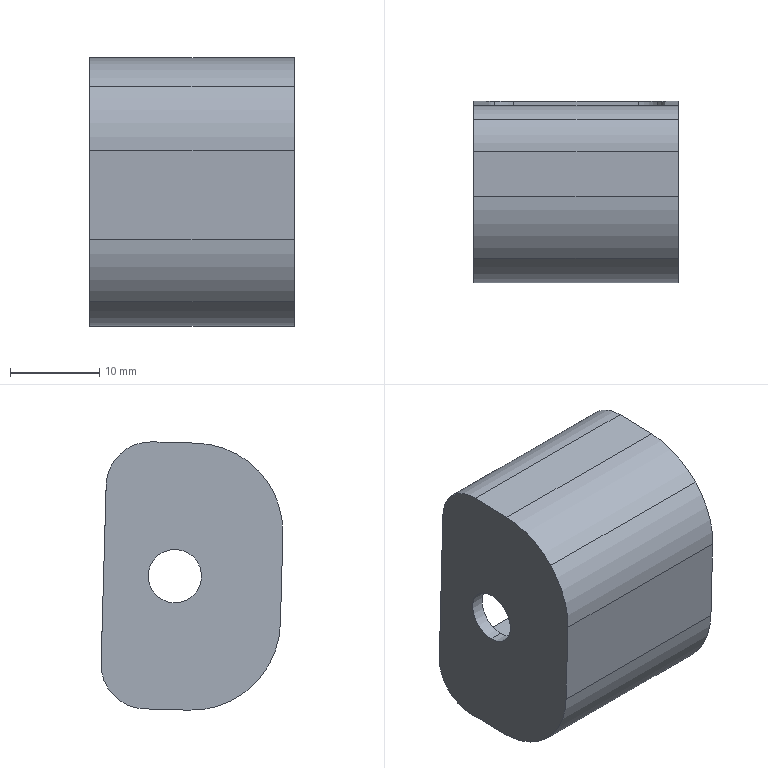Part | SolidWorks | features BaseBody 1 | 1 solid | 32 faces | box 23 x 20.424 x 30.136 mm | volume 5420 mm3 | cylinder 20 | plane 12 | commonest cylinder face diameters 6 x12 10 x4 20 x4
STEP:
#1=CARTESIAN_POINT('',(-20.895,-36.073,-245.05));
#2=VERTEX_POINT('',#1);
#3=CARTESIAN_POINT('',(-21.773,-36.013,-247.171));
#4=VERTEX_POINT('',#3);
#5=CARTESIAN_POINT('',(-18.773,-36.013,-247.171));
#6=DIRECTION('',(0.,-0.9996,-0.02838));
#7=DIRECTION('',(-0.7071,-0.02007,0.7068));
#8=AXIS2_PLACEMENT_3D('',#5,#6,#7);
#9=CIRCLE('',#8,3.);
#10=EDGE_CURVE('',#2,#4,#9,.T.);
#11=ORIENTED_EDGE('',*,*,#10,.F.);
#12=CARTESIAN_POINT('',(-20.895,-54.066,-245.561));
#13=VERTEX_POINT('',#12);
#14=CARTESIAN_POINT('',(-20.895,-36.073,-245.05));
#15=DIRECTION('',(0.,-0.9996,-0.02838));
#16=VECTOR('',#15,1000.);
#17=LINE('',#14,#16);
#18=EDGE_CURVE('',#2,#13,#17,.T.);
#19=ORIENTED_EDGE('',*,*,#18,.T.);
#20=CARTESIAN_POINT('',(-21.773,-54.005,-247.682));
#21=VERTEX_POINT('',#20);
#22=CARTESIAN_POINT('',(-18.773,-54.005,-247.682));
#23=DIRECTION('',(0.,0.9996,0.02838));
#24=DIRECTION('',(-0.7071,-0.02007,0.7068));
#25=AXIS2_PLACEMENT_3D('',#22,#23,#24);
#26=CIRCLE('',#25,3.);
#27=EDGE_CURVE('',#21,#13,#26,.T.);
#28=ORIENTED_EDGE('',*,*,#27,.F.);
#29=CARTESIAN_POINT('',(-21.773,-36.013,-247.171));
#30=DIRECTION('',(0.,0.9996,0.02838));
#31=VECTOR('',#30,1000.);
#32=LINE('',#29,#31);
#33=EDGE_CURVE('',#21,#4,#32,.T.);
#34=ORIENTED_EDGE('',*,*,#33,.T.);
#35=EDGE_LOOP('',(#11,#19,#28,#34));
#36=FACE_OUTER_BOUND('',#35,.T.);
#37=CARTESIAN_POINT('',(-18.773,-36.013,-247.171));
#38=DIRECTION('',(0.,-0.9996,-0.02838));
#39=DIRECTION('',(-0.7071,-0.02007,0.7068));
#40=AXIS2_PLACEMENT_3D('',#37,#38,#39);
#41=CYLINDRICAL_SURFACE('',#40,3.);
#42=ADVANCED_FACE('',(#36),#41,.F.);
#43=CARTESIAN_POINT('',(-2.652,-36.073,-245.05));
#44=VERTEX_POINT('',#43);
#45=CARTESIAN_POINT('',(-4.773,-36.098,-244.172));
#46=VERTEX_POINT('',#45);
#47=CARTESIAN_POINT('',(-4.773,-36.013,-247.171));
#48=DIRECTION('',(0.,-0.9996,-0.02838));
#49=DIRECTION('',(0.7071,-0.02007,0.7068));
#50=AXIS2_PLACEMENT_3D('',#47,#48,#49);
#51=CIRCLE('',#50,3.);
#52=EDGE_CURVE('',#44,#46,#51,.T.);
#53=ORIENTED_EDGE('',*,*,#52,.F.);
#54=CARTESIAN_POINT('',(-2.652,-54.066,-245.561));
#55=VERTEX_POINT('',#54);
#56=CARTESIAN_POINT('',(-2.652,-36.073,-245.05));
#57=DIRECTION('',(0.,-0.9996,-0.02838));
#58=VECTOR('',#57,1000.);
#59=LINE('',#56,#58);
#60=EDGE_CURVE('',#44,#55,#59,.T.);
#61=ORIENTED_EDGE('',*,*,#60,.T.);
#62=CARTESIAN_POINT('',(-4.773,-54.091,-244.683));
#63=VERTEX_POINT('',#62);
#64=CARTESIAN_POINT('',(-4.773,-54.005,-247.682));
#65=DIRECTION('',(0.,0.9996,0.02838));
#66=DIRECTION('',(0.7071,-0.02007,0.7068));
#67=AXIS2_PLACEMENT_3D('',#64,#65,#66);
#68=CIRCLE('',#67,3.);
#69=EDGE_CURVE('',#63,#55,#68,.T.);
#70=ORIENTED_EDGE('',*,*,#69,.F.);
#71=CARTESIAN_POINT('',(-4.773,-36.098,-244.172));
#72=DIRECTION('',(0.,0.9996,0.02838));
#73=VECTOR('',#72,1000.);
#74=LINE('',#71,#73);
#75=EDGE_CURVE('',#63,#46,#74,.T.);
#76=ORIENTED_EDGE('',*,*,#75,.T.);
#77=EDGE_LOOP('',(#53,#61,#70,#76));
#78=FACE_OUTER_BOUND('',#77,.T.);
#79=CARTESIAN_POINT('',(-4.773,-36.013,-247.171));
#80=DIRECTION('',(0.,-0.9996,-0.02838));
#81=DIRECTION('',(0.7071,-0.02007,0.7068));
#82=AXIS2_PLACEMENT_3D('',#79,#80,#81);
#83=CYLINDRICAL_SURFACE('',#82,3.);
#84=ADVANCED_FACE('',(#78),#83,.F.);
#85=CARTESIAN_POINT('',(-2.652,-35.555,-263.286));
#86=VERTEX_POINT('',#85);
#87=CARTESIAN_POINT('',(-1.773,-35.615,-261.165));
#88=VERTEX_POINT('',#87);
#89=CARTESIAN_POINT('',(-4.773,-35.615,-261.165));
#90=DIRECTION('',(0.,-0.9996,-0.02838));
#91=DIRECTION('',(0.7071,0.02007,-0.7068));
#92=AXIS2_PLACEMENT_3D('',#89,#90,#91);
#93=CIRCLE('',#92,3.);
#94=EDGE_CURVE('',#86,#88,#93,.T.);
#95=ORIENTED_EDGE('',*,*,#94,.F.);
#96=CARTESIAN_POINT('',(-2.652,-53.548,-263.797));
#97=VERTEX_POINT('',#96);
#98=CARTESIAN_POINT('',(-2.652,-35.555,-263.286));
#99=DIRECTION('',(0.,-0.9996,-0.02838));
#100=VECTOR('',#99,1000.);
#101=LINE('',#98,#100);
#102=EDGE_CURVE('',#86,#97,#101,.T.);
#103=ORIENTED_EDGE('',*,*,#102,.T.);
#104=CARTESIAN_POINT('',(-1.773,-53.608,-261.676));
#105=VERTEX_POINT('',#104);
#106=CARTESIAN_POINT('',(-4.773,-53.608,-261.676));
#107=DIRECTION('',(0.,0.9996,0.02838));
#108=DIRECTION('',(0.7071,0.02007,-0.7068));
#109=AXIS2_PLACEMENT_3D('',#106,#107,#108);
#110=CIRCLE('',#109,3.);
#111=EDGE_CURVE('',#105,#97,#110,.T.);
#112=ORIENTED_EDGE('',*,*,#111,.F.);
#113=CARTESIAN_POINT('',(-1.773,-35.615,-261.165));
#114=DIRECTION('',(0.,0.9996,0.02838));
#115=VECTOR('',#114,1000.);
#116=LINE('',#113,#115);
#117=EDGE_CURVE('',#105,#88,#116,.T.);
#118=ORIENTED_EDGE('',*,*,#117,.T.);
#119=EDGE_LOOP('',(#95,#103,#112,#118));
#120=FACE_OUTER_BOUND('',#119,.T.);
#121=CARTESIAN_POINT('',(-4.773,-35.615,-261.165));
#122=DIRECTION('',(0.,-0.9996,-0.02838));
#123=DIRECTION('',(0.7071,0.02007,-0.7068));
#124=AXIS2_PLACEMENT_3D('',#121,#122,#123);
#125=CYLINDRICAL_SURFACE('',#124,3.);
#126=ADVANCED_FACE('',(#120),#125,.F.);
#127=CARTESIAN_POINT('',(-20.895,-35.555,-263.286));
#128=VERTEX_POINT('',#127);
#129=CARTESIAN_POINT('',(-18.773,-35.53,-264.164));
#130=VERTEX_POINT('',#129);
#131=CARTESIAN_POINT('',(-18.773,-35.615,-261.165));
#132=DIRECTION('',(0.,-0.9996,-0.02838));
#133=DIRECTION('',(-0.7071,0.02007,-0.7068));
#134=AXIS2_PLACEMENT_3D('',#131,#132,#133);
#135=CIRCLE('',#134,3.);
#136=EDGE_CURVE('',#128,#130,#135,.T.);
#137=ORIENTED_EDGE('',*,*,#136,.F.);
#138=CARTESIAN_POINT('',(-20.895,-53.548,-263.797));
#139=VERTEX_POINT('',#138);
#140=CARTESIAN_POINT('',(-20.895,-35.555,-263.286));
#141=DIRECTION('',(0.,-0.9996,-0.02838));
#142=VECTOR('',#141,1000.);
#143=LINE('',#140,#142);
#144=EDGE_CURVE('',#128,#139,#143,.T.);
#145=ORIENTED_EDGE('',*,*,#144,.T.);
#146=CARTESIAN_POINT('',(-18.773,-53.523,-264.675));
#147=VERTEX_POINT('',#146);
#148=CARTESIAN_POINT('',(-18.773,-53.608,-261.676));
#149=DIRECTION('',(0.,0.9996,0.02838));
#150=DIRECTION('',(-0.7071,0.02007,-0.7068));
#151=AXIS2_PLACEMENT_3D('',#148,#149,#150);
#152=CIRCLE('',#151,3.);
#153=EDGE_CURVE('',#147,#139,#152,.T.);
#154=ORIENTED_EDGE('',*,*,#153,.F.);
#155=CARTESIAN_POINT('',(-18.773,-35.53,-264.164));
#156=DIRECTION('',(0.,0.9996,0.02838));
#157=VECTOR('',#156,1000.);
#158=LINE('',#155,#157);
#159=EDGE_CURVE('',#147,#130,#158,.T.);
#160=ORIENTED_EDGE('',*,*,#159,.T.);
#161=EDGE_LOOP('',(#137,#145,#154,#160));
#162=FACE_OUTER_BOUND('',#161,.T.);
#163=CARTESIAN_POINT('',(-18.773,-35.615,-261.165));
#164=DIRECTION('',(0.,-0.9996,-0.02838));
#165=DIRECTION('',(-0.7071,0.02007,-0.7068));
#166=AXIS2_PLACEMENT_3D('',#163,#164,#165);
#167=CYLINDRICAL_SURFACE('',#166,3.);
#168=ADVANCED_FACE('',(#162),#167,.F.);
#169=CARTESIAN_POINT('',(-0.2734,-43.726,-257.394));
#170=VERTEX_POINT('',#169);
#171=CARTESIAN_POINT('',(-0.2734,-43.896,-251.396));
#172=VERTEX_POINT('',#171);
#173=CARTESIAN_POINT('',(-0.2734,-43.811,-254.395));
#174=DIRECTION('',(-1.,0.,0.));
#175=DIRECTION('',(0.,-0.02838,0.9996));
#176=AXIS2_PLACEMENT_3D('',#173,#174,#175);
#177=CIRCLE('',#176,3.);
#178=EDGE_CURVE('',#170,#172,#177,.T.);
#179=ORIENTED_EDGE('',*,*,#178,.F.);
#180=CARTESIAN_POINT('',(-1.773,-43.726,-257.394));
#181=VERTEX_POINT('',#180);
#182=CARTESIAN_POINT('',(-0.2734,-43.726,-257.394));
#183=DIRECTION('',(-1.,0.,0.));
#184=VECTOR('',#183,1000.);
#185=LINE('',#182,#184);
#186=EDGE_CURVE('',#170,#181,#185,.T.);
#187=ORIENTED_EDGE('',*,*,#186,.T.);
#188=CARTESIAN_POINT('',(-1.773,-43.896,-251.396));
#189=VERTEX_POINT('',#188);
#190=CARTESIAN_POINT('',(-1.773,-43.811,-254.395));
#191=DIRECTION('',(1.,0.,0.));
#192=DIRECTION('',(0.,-0.02838,0.9996));
#193=AXIS2_PLACEMENT_3D('',#190,#191,#192);
#194=CIRCLE('',#193,3.);
#195=EDGE_CURVE('',#189,#181,#194,.T.);
#196=ORIENTED_EDGE('',*,*,#195,.F.);
#197=CARTESIAN_POINT('',(-0.2734,-43.896,-251.396));
#198=DIRECTION('',(-1.,0.,0.));
#199=VECTOR('',#198,1000.);
#200=LINE('',#197,#199);
#201=EDGE_CURVE('',#172,#189,#200,.T.);
#202=ORIENTED_EDGE('',*,*,#201,.F.);
#203=EDGE_LOOP('',(#179,#187,#196,#202));
#204=FACE_OUTER_BOUND('',#203,.T.);
#205=CARTESIAN_POINT('',(-0.2734,-43.811,-254.395));
#206=DIRECTION('',(-1.,0.,0.));
#207=DIRECTION('',(0.,-0.02838,0.9996));
#208=AXIS2_PLACEMENT_3D('',#205,#206,#207);
#209=CYLINDRICAL_SURFACE('',#208,3.);
#210=ADVANCED_FACE('',(#204),#209,.F.);
#211=CARTESIAN_POINT('',(-21.773,-43.726,-257.394));
#212=VERTEX_POINT('',#211);
#213=CARTESIAN_POINT('',(-21.773,-43.896,-251.396));
#214=VERTEX_POINT('',#213);
#215=CARTESIAN_POINT('',(-21.773,-43.811,-254.395));
#216=DIRECTION('',(-1.,0.,0.));
#217=DIRECTION('',(0.,-0.02838,0.9996));
#218=AXIS2_PLACEMENT_3D('',#215,#216,#217);
#219=CIRCLE('',#218,3.);
#220=EDGE_CURVE('',#212,#214,#219,.T.);
#221=ORIENTED_EDGE('',*,*,#220,.F.);
#222=CARTESIAN_POINT('',(-23.273,-43.726,-257.394));
#223=VERTEX_POINT('',#222);
#224=CARTESIAN_POINT('',(-0.2734,-43.726,-257.394));
#225=DIRECTION('',(-1.,0.,0.));
#226=VECTOR('',#225,1000.);
#227=LINE('',#224,#226);
#228=EDGE_CURVE('',#212,#223,#227,.T.);
#229=ORIENTED_EDGE('',*,*,#228,.T.);
#230=CARTESIAN_POINT('',(-23.273,-43.896,-251.396));
#231=VERTEX_POINT('',#230);
#232=CARTESIAN_POINT('',(-23.273,-43.811,-254.395));
#233=DIRECTION('',(1.,0.,0.));
#234=DIRECTION('',(0.,-0.02838,0.9996));
#235=AXIS2_PLACEMENT_3D('',#232,#233,#234);
#236=CIRCLE('',#235,3.);
#237=EDGE_CURVE('',#231,#223,#236,.T.);
#238=ORIENTED_EDGE('',*,*,#237,.F.);
#239=CARTESIAN_POINT('',(-0.2734,-43.896,-251.396));
#240=DIRECTION('',(-1.,0.,0.));
#241=VECTOR('',#240,1000.);
#242=LINE('',#239,#241);
#243=EDGE_CURVE('',#214,#231,#242,.T.);
#244=ORIENTED_EDGE('',*,*,#243,.F.);
#245=EDGE_LOOP('',(#221,#229,#238,#244));
#246=FACE_OUTER_BOUND('',#245,.T.);
#247=CARTESIAN_POINT('',(-0.2734,-43.811,-254.395));
#248=DIRECTION('',(-1.,0.,0.));
#249=DIRECTION('',(0.,-0.02838,0.9996));
#250=AXIS2_PLACEMENT_3D('',#247,#248,#249);
#251=CYLINDRICAL_SURFACE('',#250,3.);
#252=ADVANCED_FACE('',(#246),#251,.F.);
#253=CARTESIAN_POINT('',(-0.2734,-55.948,-249.738));
#254=VERTEX_POINT('',#253);
#255=CARTESIAN_POINT('',(-0.2734,-53.221,-242.586));
#256=VERTEX_POINT('',#255);
#257=CARTESIAN_POINT('',(-0.2734,-45.952,-249.454));
#258=DIRECTION('',(-1.,0.,0.));
#259=DIRECTION('',(0.,-0.7269,0.6868));
#260=AXIS2_PLACEMENT_3D('',#257,#258,#259);
#261=CIRCLE('',#260,10.);
#262=EDGE_CURVE('',#254,#256,#261,.T.);
#263=ORIENTED_EDGE('',*,*,#262,.T.);
#264=CARTESIAN_POINT('',(-23.273,-53.221,-242.586));
#265=VERTEX_POINT('',#264);
#266=CARTESIAN_POINT('',(-11.773,-53.221,-242.586));
#267=DIRECTION('',(-1.,0.,0.));
#268=VECTOR('',#267,1000.);
#269=LINE('',#266,#268);
#270=EDGE_CURVE('',#256,#265,#269,.T.);
#271=ORIENTED_EDGE('',*,*,#270,.T.);
#272=CARTESIAN_POINT('',(-23.273,-55.948,-249.738));
#273=VERTEX_POINT('',#272);
#274=CARTESIAN_POINT('',(-23.273,-45.952,-249.454));
#275=DIRECTION('',(1.,0.,0.));
#276=DIRECTION('',(0.,-0.7269,0.6868));
#277=AXIS2_PLACEMENT_3D('',#274,#275,#276);
#278=CIRCLE('',#277,10.);
#279=EDGE_CURVE('',#265,#273,#278,.T.);
#280=ORIENTED_EDGE('',*,*,#279,.T.);
#281=CARTESIAN_POINT('',(-11.773,-55.948,-249.738));
#282=DIRECTION('',(1.,0.,0.));
#283=VECTOR('',#282,1000.);
#284=LINE('',#281,#283);
#285=EDGE_CURVE('',#273,#254,#284,.T.);
#286=ORIENTED_EDGE('',*,*,#285,.T.);
#287=EDGE_LOOP('',(#263,#271,#280,#286));
#288=FACE_OUTER_BOUND('',#287,.T.);
#289=CARTESIAN_POINT('',(-11.773,-45.952,-249.454));
#290=DIRECTION('',(-1.,0.,0.));
#291=DIRECTION('',(0.,-0.7269,0.6868));
#292=AXIS2_PLACEMENT_3D('',#289,#290,#291);
#293=CYLINDRICAL_SURFACE('',#292,10.);
#294=ADVANCED_FACE('',(#288),#293,.T.);
#295=CARTESIAN_POINT('',(-0.2734,-45.384,-269.446));
#296=VERTEX_POINT('',#295);
#297=CARTESIAN_POINT('',(-0.2734,-52.536,-266.719));
#298=VERTEX_POINT('',#297);
#299=CARTESIAN_POINT('',(-0.2734,-45.668,-259.45));
#300=DIRECTION('',(-1.,0.,0.));
#301=DIRECTION('',(0.,-0.6868,-0.7269));
#302=AXIS2_PLACEMENT_3D('',#299,#300,#301);
#303=CIRCLE('',#302,10.);
#304=EDGE_CURVE('',#296,#298,#303,.T.);
#305=ORIENTED_EDGE('',*,*,#304,.T.);
#306=CARTESIAN_POINT('',(-23.273,-52.536,-266.719));
#307=VERTEX_POINT('',#306);
#308=CARTESIAN_POINT('',(-11.773,-52.536,-266.719));
#309=DIRECTION('',(-1.,0.,0.));
#310=VECTOR('',#309,1000.);
#311=LINE('',#308,#310);
#312=EDGE_CURVE('',#298,#307,#311,.T.);
#313=ORIENTED_EDGE('',*,*,#312,.T.);
#314=CARTESIAN_POINT('',(-23.273,-45.384,-269.446));
#315=VERTEX_POINT('',#314);
#316=CARTESIAN_POINT('',(-23.273,-45.668,-259.45));
#317=DIRECTION('',(1.,0.,0.));
#318=DIRECTION('',(0.,-0.6868,-0.7269));
#319=AXIS2_PLACEMENT_3D('',#316,#317,#318);
#320=CIRCLE('',#319,10.);
#321=EDGE_CURVE('',#307,#315,#320,.T.);
#322=ORIENTED_EDGE('',*,*,#321,.T.);
#323=CARTESIAN_POINT('',(-11.773,-45.384,-269.446));
#324=DIRECTION('',(1.,0.,0.));
#325=VECTOR('',#324,1000.);
#326=LINE('',#323,#325);
#327=EDGE_CURVE('',#315,#296,#326,.T.);
#328=ORIENTED_EDGE('',*,*,#327,.T.);
#329=EDGE_LOOP('',(#305,#313,#322,#328));
#330=FACE_OUTER_BOUND('',#329,.T.);
#331=CARTESIAN_POINT('',(-11.773,-45.668,-259.45));
#332=DIRECTION('',(-1.,0.,0.));
#333=DIRECTION('',(0.,-0.6868,-0.7269));
#334=AXIS2_PLACEMENT_3D('',#331,#332,#333);
#335=CYLINDRICAL_SURFACE('',#334,10.);
#336=ADVANCED_FACE('',(#330),#335,.T.);
#337=CARTESIAN_POINT('',(-23.273,-36.098,-244.172));
#338=VERTEX_POINT('',#337);
#339=CARTESIAN_POINT('',(-23.273,-37.662,-240.68));
#340=VERTEX_POINT('',#339);
#341=CARTESIAN_POINT('',(-23.273,-41.096,-244.314));
#342=DIRECTION('',(1.,0.,0.));
#343=DIRECTION('',(0.,0.6868,0.7269));
#344=AXIS2_PLACEMENT_3D('',#341,#342,#343);
#345=CIRCLE('',#344,5.);
#346=EDGE_CURVE('',#338,#340,#345,.T.);
#347=ORIENTED_EDGE('',*,*,#346,.T.);
#348=CARTESIAN_POINT('',(-0.2734,-37.662,-240.68));
#349=VERTEX_POINT('',#348);
#350=CARTESIAN_POINT('',(-11.773,-37.662,-240.68));
#351=DIRECTION('',(1.,0.,0.));
#352=VECTOR('',#351,1000.);
#353=LINE('',#350,#352);
#354=EDGE_CURVE('',#340,#349,#353,.T.);
#355=ORIENTED_EDGE('',*,*,#354,.T.);
#356=CARTESIAN_POINT('',(-0.2734,-36.098,-244.172));
#357=VERTEX_POINT('',#356);
#358=CARTESIAN_POINT('',(-0.2734,-41.096,-244.314));
#359=DIRECTION('',(-1.,0.,0.));
#360=DIRECTION('',(0.,0.6868,0.7269));
#361=AXIS2_PLACEMENT_3D('',#358,#359,#360);
#362=CIRCLE('',#361,5.);
#363=EDGE_CURVE('',#349,#357,#362,.T.);
#364=ORIENTED_EDGE('',*,*,#363,.T.);
#365=CARTESIAN_POINT('',(-6.773,-36.098,-244.172));
#366=DIRECTION('',(-1.,0.,0.));
#367=VECTOR('',#366,1000.);
#368=LINE('',#365,#367);
#369=EDGE_CURVE('',#357,#46,#368,.T.);
#370=ORIENTED_EDGE('',*,*,#369,.T.);
#371=CARTESIAN_POINT('',(-18.773,-36.098,-244.172));
#372=VERTEX_POINT('',#371);
#373=CARTESIAN_POINT('',(-6.773,-36.098,-244.172));
#374=DIRECTION('',(-1.,0.,0.));
#375=VECTOR('',#374,1000.);
#376=LINE('',#373,#375);
#377=EDGE_CURVE('',#46,#372,#376,.T.);
#378=ORIENTED_EDGE('',*,*,#377,.T.);
#379=CARTESIAN_POINT('',(-6.773,-36.098,-244.172));
#380=DIRECTION('',(-1.,0.,0.));
#381=VECTOR('',#380,1000.);
#382=LINE('',#379,#381);
#383=EDGE_CURVE('',#372,#338,#382,.T.);
#384=ORIENTED_EDGE('',*,*,#383,.T.);
#385=EDGE_LOOP('',(#347,#355,#364,#370,#378,#384));
#386=FACE_OUTER_BOUND('',#385,.T.);
#387=CARTESIAN_POINT('',(-11.773,-41.096,-244.314));
#388=DIRECTION('',(1.,0.,0.));
#389=DIRECTION('',(0.,0.6868,0.7269));
#390=AXIS2_PLACEMENT_3D('',#387,#388,#389);
#391=CYLINDRICAL_SURFACE('',#390,5.);
#392=ADVANCED_FACE('',(#386),#391,.T.);
#393=CARTESIAN_POINT('',(-0.2734,-35.53,-264.164));
#394=VERTEX_POINT('',#393);
#395=CARTESIAN_POINT('',(-0.2734,-36.894,-267.74));
#396=VERTEX_POINT('',#395);
#397=CARTESIAN_POINT('',(-0.2734,-40.528,-264.306));
#398=DIRECTION('',(-1.,0.,0.));
#399=DIRECTION('',(0.,0.7269,-0.6868));
#400=AXIS2_PLACEMENT_3D('',#397,#398,#399);
#401=CIRCLE('',#400,5.);
#402=EDGE_CURVE('',#394,#396,#401,.T.);
#403=ORIENTED_EDGE('',*,*,#402,.T.);
#404=CARTESIAN_POINT('',(-23.273,-36.894,-267.74));
#405=VERTEX_POINT('',#404);
#406=CARTESIAN_POINT('',(-11.773,-36.894,-267.74));
#407=DIRECTION('',(-1.,0.,0.));
#408=VECTOR('',#407,1000.);
#409=LINE('',#406,#408);
#410=EDGE_CURVE('',#396,#405,#409,.T.);
#411=ORIENTED_EDGE('',*,*,#410,.T.);
#412=CARTESIAN_POINT('',(-23.273,-35.53,-264.164));
#413=VERTEX_POINT('',#412);
#414=CARTESIAN_POINT('',(-23.273,-40.528,-264.306));
#415=DIRECTION('',(1.,0.,0.));
#416=DIRECTION('',(0.,0.7269,-0.6868));
#417=AXIS2_PLACEMENT_3D('',#414,#415,#416);
#418=CIRCLE('',#417,5.);
#419=EDGE_CURVE('',#405,#413,#418,.T.);
#420=ORIENTED_EDGE('',*,*,#419,.T.);
#421=CARTESIAN_POINT('',(-16.773,-35.53,-264.164));
#422=DIRECTION('',(1.,0.,0.));
#423=VECTOR('',#422,1000.);
#424=LINE('',#421,#423);
#425=EDGE_CURVE('',#413,#130,#424,.T.);
#426=ORIENTED_EDGE('',*,*,#425,.T.);
#427=CARTESIAN_POINT('',(-4.773,-35.53,-264.164));
#428=VERTEX_POINT('',#427);
#429=CARTESIAN_POINT('',(-16.773,-35.53,-264.164));
#430=DIRECTION('',(1.,0.,0.));
#431=VECTOR('',#430,1000.);
#432=LINE('',#429,#431);
#433=EDGE_CURVE('',#130,#428,#432,.T.);
#434=ORIENTED_EDGE('',*,*,#433,.T.);
#435=CARTESIAN_POINT('',(-16.773,-35.53,-264.164));
#436=DIRECTION('',(1.,0.,0.));
#437=VECTOR('',#436,1000.);
#438=LINE('',#435,#437);
#439=EDGE_CURVE('',#428,#394,#438,.T.);
#440=ORIENTED_EDGE('',*,*,#439,.T.);
#441=EDGE_LOOP('',(#403,#411,#420,#426,#434,#440));
#442=FACE_OUTER_BOUND('',#441,.T.);
#443=CARTESIAN_POINT('',(-11.773,-40.528,-264.306));
#444=DIRECTION('',(-1.,0.,0.));
#445=DIRECTION('',(0.,0.7269,-0.6868));
#446=AXIS2_PLACEMENT_3D('',#443,#444,#445);
#447=CYLINDRICAL_SURFACE('',#446,5.);
#448=ADVANCED_FACE('',(#442),#447,.T.);
#449=CARTESIAN_POINT('',(-0.2734,-43.811,-254.395));
#450=DIRECTION('',(-1.,0.,0.));
#451=DIRECTION('',(0.,-0.02838,0.9996));
#452=AXIS2_PLACEMENT_3D('',#449,#450,#451);
#453=CIRCLE('',#452,3.);
#454=EDGE_CURVE('',#172,#170,#453,.T.);
#455=ORIENTED_EDGE('',*,*,#454,.T.);
#456=ORIENTED_EDGE('',*,*,#178,.T.);
#457=EDGE_LOOP('',(#455,#456));
#458=FACE_BOUND('',#457,.T.);
#459=ORIENTED_EDGE('',*,*,#262,.F.);
#460=CARTESIAN_POINT('',(-0.2734,-55.664,-259.734));
#461=VERTEX_POINT('',#460);
#462=CARTESIAN_POINT('',(-0.2734,-55.38,-269.73));
#463=DIRECTION('',(0.,0.02838,-0.9996));
#464=VECTOR('',#463,1000.);
#465=LINE('',#462,#464);
#466=EDGE_CURVE('',#254,#461,#465,.T.);
#467=ORIENTED_EDGE('',*,*,#466,.T.);
#468=CARTESIAN_POINT('',(-0.2734,-45.668,-259.45));
#469=DIRECTION('',(-1.,0.,0.));
#470=DIRECTION('',(0.,-0.6868,-0.7269));
#471=AXIS2_PLACEMENT_3D('',#468,#469,#470);
#472=CIRCLE('',#471,10.);
#473=EDGE_CURVE('',#298,#461,#472,.T.);
#474=ORIENTED_EDGE('',*,*,#473,.F.);
#475=ORIENTED_EDGE('',*,*,#304,.F.);
#476=CARTESIAN_POINT('',(-0.2734,-40.386,-269.304));
#477=VERTEX_POINT('',#476);
#478=CARTESIAN_POINT('',(-0.2734,-35.388,-269.162));
#479=DIRECTION('',(0.,0.9996,0.02838));
#480=VECTOR('',#479,1000.);
#481=LINE('',#478,#480);
#482=EDGE_CURVE('',#296,#477,#481,.T.);
#483=ORIENTED_EDGE('',*,*,#482,.T.);
#484=CARTESIAN_POINT('',(-0.2734,-40.528,-264.306));
#485=DIRECTION('',(-1.,0.,0.));
#486=DIRECTION('',(0.,0.7269,-0.6868));
#487=AXIS2_PLACEMENT_3D('',#484,#485,#486);
#488=CIRCLE('',#487,5.);
#489=EDGE_CURVE('',#396,#477,#488,.T.);
#490=ORIENTED_EDGE('',*,*,#489,.F.);
#491=ORIENTED_EDGE('',*,*,#402,.F.);
#492=CARTESIAN_POINT('',(-0.2734,-36.24,-239.174));
#493=DIRECTION('',(0.,-0.02838,0.9996));
#494=VECTOR('',#493,1000.);
#495=LINE('',#492,#494);
#496=EDGE_CURVE('',#394,#357,#495,.T.);
#497=ORIENTED_EDGE('',*,*,#496,.T.);
#498=ORIENTED_EDGE('',*,*,#363,.F.);
#499=CARTESIAN_POINT('',(-0.2734,-41.238,-239.316));
#500=VERTEX_POINT('',#499);
#501=CARTESIAN_POINT('',(-0.2734,-41.096,-244.314));
#502=DIRECTION('',(-1.,0.,0.));
#503=DIRECTION('',(0.,0.6868,0.7269));
#504=AXIS2_PLACEMENT_3D('',#501,#502,#503);
#505=CIRCLE('',#504,5.);
#506=EDGE_CURVE('',#500,#349,#505,.T.);
#507=ORIENTED_EDGE('',*,*,#506,.F.);
#508=CARTESIAN_POINT('',(-0.2734,-46.236,-239.458));
#509=VERTEX_POINT('',#508);
#510=CARTESIAN_POINT('',(-0.2734,-56.232,-239.742));
#511=DIRECTION('',(0.,-0.9996,-0.02838));
#512=VECTOR('',#511,1000.);
#513=LINE('',#510,#512);
#514=EDGE_CURVE('',#500,#509,#513,.T.);
#515=ORIENTED_EDGE('',*,*,#514,.T.);
#516=CARTESIAN_POINT('',(-0.2734,-45.952,-249.454));
#517=DIRECTION('',(-1.,0.,0.));
#518=DIRECTION('',(0.,-0.7269,0.6868));
#519=AXIS2_PLACEMENT_3D('',#516,#517,#518);
#520=CIRCLE('',#519,10.);
#521=EDGE_CURVE('',#256,#509,#520,.T.);
#522=ORIENTED_EDGE('',*,*,#521,.F.);
#523=EDGE_LOOP('',(#459,#467,#474,#475,#483,#490,#491,#497,#498,#507,#515,#522));
#524=FACE_OUTER_BOUND('',#523,.T.);
#525=CARTESIAN_POINT('',(-0.2734,-45.81,-254.452));
#526=DIRECTION('',(1.,0.,0.));
#527=DIRECTION('',(0.,0.02838,-0.9996));
#528=AXIS2_PLACEMENT_3D('',#525,#526,#527);
#529=PLANE('',#528);
#530=ADVANCED_FACE('',(#458,#524),#529,.T.);
#531=CARTESIAN_POINT('',(-23.273,-46.236,-239.458));
#532=VERTEX_POINT('',#531);
#533=CARTESIAN_POINT('',(-11.773,-46.236,-239.458));
#534=DIRECTION('',(-1.,0.,0.));
#535=VECTOR('',#534,1000.);
#536=LINE('',#533,#535);
#537=EDGE_CURVE('',#509,#532,#536,.T.);
#538=ORIENTED_EDGE('',*,*,#537,.F.);
#539=ORIENTED_EDGE('',*,*,#514,.F.);
#540=CARTESIAN_POINT('',(-23.273,-41.238,-239.316));
#541=VERTEX_POINT('',#540);
#542=CARTESIAN_POINT('',(-11.773,-41.238,-239.316));
#543=DIRECTION('',(1.,0.,0.));
#544=VECTOR('',#543,1000.);
#545=LINE('',#542,#544);
#546=EDGE_CURVE('',#541,#500,#545,.T.);
#547=ORIENTED_EDGE('',*,*,#546,.F.);
#548=CARTESIAN_POINT('',(-23.273,-56.232,-239.742));
#549=DIRECTION('',(0.,0.9996,0.02838));
#550=VECTOR('',#549,1000.);
#551=LINE('',#548,#550);
#552=EDGE_CURVE('',#532,#541,#551,.T.);
#553=ORIENTED_EDGE('',*,*,#552,.F.);
#554=EDGE_LOOP('',(#538,#539,#547,#553));
#555=FACE_OUTER_BOUND('',#554,.T.);
#556=CARTESIAN_POINT('',(-11.773,-36.24,-239.174));
#557=DIRECTION('',(0.,-0.02838,0.9996));
#558=DIRECTION('',(0.,0.9996,0.02838));
#559=AXIS2_PLACEMENT_3D('',#556,#557,#558);
#560=PLANE('',#559);
#561=ADVANCED_FACE('',(#555),#560,.T.);
#562=ORIENTED_EDGE('',*,*,#195,.T.);
#563=CARTESIAN_POINT('',(-1.773,-43.811,-254.395));
#564=DIRECTION('',(1.,0.,0.));
#565=DIRECTION('',(0.,-0.02838,0.9996));
#566=AXIS2_PLACEMENT_3D('',#563,#564,#565);
#567=CIRCLE('',#566,3.);
#568=EDGE_CURVE('',#181,#189,#567,.T.);
#569=ORIENTED_EDGE('',*,*,#568,.T.);
#570=EDGE_LOOP('',(#562,#569));
#571=FACE_BOUND('',#570,.T.);
#572=CARTESIAN_POINT('',(-1.773,-36.013,-247.171));
#573=VERTEX_POINT('',#572);
#574=CARTESIAN_POINT('',(-1.773,-54.005,-247.682));
#575=VERTEX_POINT('',#574);
#576=CARTESIAN_POINT('',(-1.773,-36.013,-247.171));
#577=DIRECTION('',(0.,-0.9996,-0.02838));
#578=VECTOR('',#577,1000.);
#579=LINE('',#576,#578);
#580=EDGE_CURVE('',#573,#575,#579,.T.);
#581=ORIENTED_EDGE('',*,*,#580,.F.);
#582=CARTESIAN_POINT('',(-1.773,-35.459,-266.663));
#583=DIRECTION('',(0.,-0.02838,0.9996));
#584=VECTOR('',#583,1000.);
#585=LINE('',#582,#584);
#586=EDGE_CURVE('',#88,#573,#585,.T.);
#587=ORIENTED_EDGE('',*,*,#586,.F.);
#588=ORIENTED_EDGE('',*,*,#117,.F.);
#589=CARTESIAN_POINT('',(-1.773,-54.091,-244.683));
#590=DIRECTION('',(0.,-0.02838,0.9996));
#591=VECTOR('',#590,1000.);
#592=LINE('',#589,#591);
#593=EDGE_CURVE('',#105,#575,#592,.T.);
#594=ORIENTED_EDGE('',*,*,#593,.T.);
#595=EDGE_LOOP('',(#581,#587,#588,#594));
#596=FACE_OUTER_BOUND('',#595,.T.);
#597=CARTESIAN_POINT('',(-1.773,-35.53,-264.164));
#598=DIRECTION('',(1.,0.,0.));
#599=DIRECTION('',(0.,0.02838,-0.9996));
#600=AXIS2_PLACEMENT_3D('',#597,#598,#599);
#601=PLANE('',#600);
#602=ADVANCED_FACE('',(#571,#596),#601,.F.);
#603=ORIENTED_EDGE('',*,*,#410,.F.);
#604=ORIENTED_EDGE('',*,*,#489,.T.);
#605=CARTESIAN_POINT('',(-23.273,-40.386,-269.304));
#606=VERTEX_POINT('',#605);
#607=CARTESIAN_POINT('',(-11.773,-40.386,-269.304));
#608=DIRECTION('',(-1.,0.,0.));
#609=VECTOR('',#608,1000.);
#610=LINE('',#607,#609);
#611=EDGE_CURVE('',#477,#606,#610,.T.);
#612=ORIENTED_EDGE('',*,*,#611,.T.);
#613=CARTESIAN_POINT('',(-23.273,-40.528,-264.306));
#614=DIRECTION('',(1.,0.,0.));
#615=DIRECTION('',(0.,0.7269,-0.6868));
#616=AXIS2_PLACEMENT_3D('',#613,#614,#615);
#617=CIRCLE('',#616,5.);
#618=EDGE_CURVE('',#606,#405,#617,.T.);
#619=ORIENTED_EDGE('',*,*,#618,.T.);
#620=EDGE_LOOP('',(#603,#604,#612,#619));
#621=FACE_OUTER_BOUND('',#620,.T.);
#622=CARTESIAN_POINT('',(-11.773,-40.528,-264.306));
#623=DIRECTION('',(-1.,0.,0.));
#624=DIRECTION('',(0.,0.7269,-0.6868));
#625=AXIS2_PLACEMENT_3D('',#622,#623,#624);
#626=CYLINDRICAL_SURFACE('',#625,5.);
#627=ADVANCED_FACE('',(#621),#626,.T.);
#628=ORIENTED_EDGE('',*,*,#383,.F.);
#629=CARTESIAN_POINT('',(-18.773,-36.013,-247.171));
#630=DIRECTION('',(0.,-0.9996,-0.02838));
#631=DIRECTION('',(-0.7071,-0.02007,0.7068));
#632=AXIS2_PLACEMENT_3D('',#629,#630,#631);
#633=CIRCLE('',#632,3.);
#634=EDGE_CURVE('',#372,#2,#633,.T.);
#635=ORIENTED_EDGE('',*,*,#634,.T.);
#636=ORIENTED_EDGE('',*,*,#10,.T.);
#637=CARTESIAN_POINT('',(-21.773,-35.615,-261.165));
#638=VERTEX_POINT('',#637);
#639=CARTESIAN_POINT('',(-21.773,-35.743,-256.667));
#640=DIRECTION('',(0.,0.02838,-0.9996));
#641=VECTOR('',#640,1000.);
#642=LINE('',#639,#641);
#643=EDGE_CURVE('',#4,#638,#642,.T.);
#644=ORIENTED_EDGE('',*,*,#643,.T.);
#645=CARTESIAN_POINT('',(-18.773,-35.615,-261.165));
#646=DIRECTION('',(0.,-0.9996,-0.02838));
#647=DIRECTION('',(-0.7071,0.02007,-0.7068));
#648=AXIS2_PLACEMENT_3D('',#645,#646,#647);
#649=CIRCLE('',#648,3.);
#650=EDGE_CURVE('',#638,#128,#649,.T.);
#651=ORIENTED_EDGE('',*,*,#650,.T.);
#652=ORIENTED_EDGE('',*,*,#136,.T.);
#653=ORIENTED_EDGE('',*,*,#425,.F.);
#654=CARTESIAN_POINT('',(-23.273,-36.24,-239.174));
#655=DIRECTION('',(0.,0.02838,-0.9996));
#656=VECTOR('',#655,1000.);
#657=LINE('',#654,#656);
#658=EDGE_CURVE('',#338,#413,#657,.T.);
#659=ORIENTED_EDGE('',*,*,#658,.F.);
#660=EDGE_LOOP('',(#628,#635,#636,#644,#651,#652,#653,#659));
#661=FACE_OUTER_BOUND('',#660,.T.);
#662=CARTESIAN_POINT('',(-11.773,-35.388,-269.162));
#663=DIRECTION('',(0.,0.9996,0.02838));
#664=DIRECTION('',(0.,0.02838,-0.9996));
#665=AXIS2_PLACEMENT_3D('',#662,#663,#664);
#666=PLANE('',#665);
#667=ADVANCED_FACE('',(#661),#666,.T.);
#668=ORIENTED_EDGE('',*,*,#369,.F.);
#669=ORIENTED_EDGE('',*,*,#496,.F.);
#670=ORIENTED_EDGE('',*,*,#439,.F.);
#671=CARTESIAN_POINT('',(-4.773,-35.615,-261.165));
#672=DIRECTION('',(0.,-0.9996,-0.02838));
#673=DIRECTION('',(0.7071,0.02007,-0.7068));
#674=AXIS2_PLACEMENT_3D('',#671,#672,#673);
#675=CIRCLE('',#674,3.);
#676=EDGE_CURVE('',#428,#86,#675,.T.);
#677=ORIENTED_EDGE('',*,*,#676,.T.);
#678=ORIENTED_EDGE('',*,*,#94,.T.);
#679=ORIENTED_EDGE('',*,*,#586,.T.);
#680=CARTESIAN_POINT('',(-4.773,-36.013,-247.171));
#681=DIRECTION('',(0.,-0.9996,-0.02838));
#682=DIRECTION('',(0.7071,-0.02007,0.7068));
#683=AXIS2_PLACEMENT_3D('',#680,#681,#682);
#684=CIRCLE('',#683,3.);
#685=EDGE_CURVE('',#573,#44,#684,.T.);
#686=ORIENTED_EDGE('',*,*,#685,.T.);
#687=ORIENTED_EDGE('',*,*,#52,.T.);
#688=EDGE_LOOP('',(#668,#669,#670,#677,#678,#679,#686,#687));
#689=FACE_OUTER_BOUND('',#688,.T.);
#690=CARTESIAN_POINT('',(-11.773,-35.388,-269.162));
#691=DIRECTION('',(0.,0.9996,0.02838));
#692=DIRECTION('',(0.,0.02838,-0.9996));
#693=AXIS2_PLACEMENT_3D('',#690,#691,#692);
#694=PLANE('',#693);
#695=ADVANCED_FACE('',(#689),#694,.T.);
#696=ORIENTED_EDGE('',*,*,#354,.F.);
#697=CARTESIAN_POINT('',(-23.273,-41.096,-244.314));
#698=DIRECTION('',(1.,0.,0.));
#699=DIRECTION('',(0.,0.6868,0.7269));
#700=AXIS2_PLACEMENT_3D('',#697,#698,#699);
#701=CIRCLE('',#700,5.);
#702=EDGE_CURVE('',#340,#541,#701,.T.);
#703=ORIENTED_EDGE('',*,*,#702,.T.);
#704=ORIENTED_EDGE('',*,*,#546,.T.);
#705=ORIENTED_EDGE('',*,*,#506,.T.);
#706=EDGE_LOOP('',(#696,#703,#704,#705));
#707=FACE_OUTER_BOUND('',#706,.T.);
#708=CARTESIAN_POINT('',(-11.773,-41.096,-244.314));
#709=DIRECTION('',(1.,0.,0.));
#710=DIRECTION('',(0.,0.6868,0.7269));
#711=AXIS2_PLACEMENT_3D('',#708,#709,#710);
#712=CYLINDRICAL_SURFACE('',#711,5.);
#713=ADVANCED_FACE('',(#707),#712,.T.);
#714=ORIENTED_EDGE('',*,*,#327,.F.);
#715=CARTESIAN_POINT('',(-23.273,-35.388,-269.162));
#716=DIRECTION('',(0.,-0.9996,-0.02838));
#717=VECTOR('',#716,1000.);
#718=LINE('',#715,#717);
#719=EDGE_CURVE('',#606,#315,#718,.T.);
#720=ORIENTED_EDGE('',*,*,#719,.F.);
#721=ORIENTED_EDGE('',*,*,#611,.F.);
#722=ORIENTED_EDGE('',*,*,#482,.F.);
#723=EDGE_LOOP('',(#714,#720,#721,#722));
#724=FACE_OUTER_BOUND('',#723,.T.);
#725=CARTESIAN_POINT('',(-11.773,-55.38,-269.73));
#726=DIRECTION('',(0.,0.02838,-0.9996));
#727=DIRECTION('',(0.,0.9996,0.02838));
#728=AXIS2_PLACEMENT_3D('',#725,#726,#727);
#729=PLANE('',#728);
#730=ADVANCED_FACE('',(#724),#729,.T.);
#731=ORIENTED_EDGE('',*,*,#312,.F.);
#732=ORIENTED_EDGE('',*,*,#473,.T.);
#733=CARTESIAN_POINT('',(-23.273,-55.664,-259.734));
#734=VERTEX_POINT('',#733);
#735=CARTESIAN_POINT('',(-11.773,-55.664,-259.734));
#736=DIRECTION('',(-1.,0.,0.));
#737=VECTOR('',#736,1000.);
#738=LINE('',#735,#737);
#739=EDGE_CURVE('',#461,#734,#738,.T.);
#740=ORIENTED_EDGE('',*,*,#739,.T.);
#741=CARTESIAN_POINT('',(-23.273,-45.668,-259.45));
#742=DIRECTION('',(1.,0.,0.));
#743=DIRECTION('',(0.,-0.6868,-0.7269));
#744=AXIS2_PLACEMENT_3D('',#741,#742,#743);
#745=CIRCLE('',#744,10.);
#746=EDGE_CURVE('',#734,#307,#745,.T.);
#747=ORIENTED_EDGE('',*,*,#746,.T.);
#748=EDGE_LOOP('',(#731,#732,#740,#747));
#749=FACE_OUTER_BOUND('',#748,.T.);
#750=CARTESIAN_POINT('',(-11.773,-45.668,-259.45));
#751=DIRECTION('',(-1.,0.,0.));
#752=DIRECTION('',(0.,-0.6868,-0.7269));
#753=AXIS2_PLACEMENT_3D('',#750,#751,#752);
#754=CYLINDRICAL_SURFACE('',#753,10.);
#755=ADVANCED_FACE('',(#749),#754,.T.);
#756=ORIENTED_EDGE('',*,*,#237,.T.);
#757=CARTESIAN_POINT('',(-23.273,-43.811,-254.395));
#758=DIRECTION('',(1.,0.,0.));
#759=DIRECTION('',(0.,-0.02838,0.9996));
#760=AXIS2_PLACEMENT_3D('',#757,#758,#759);
#761=CIRCLE('',#760,3.);
#762=EDGE_CURVE('',#223,#231,#761,.T.);
#763=ORIENTED_EDGE('',*,*,#762,.T.);
#764=EDGE_LOOP('',(#756,#763));
#765=FACE_BOUND('',#764,.T.);
#766=CARTESIAN_POINT('',(-23.273,-45.952,-249.454));
#767=DIRECTION('',(1.,0.,0.));
#768=DIRECTION('',(0.,-0.7269,0.6868));
#769=AXIS2_PLACEMENT_3D('',#766,#767,#768);
#770=CIRCLE('',#769,10.);
#771=EDGE_CURVE('',#532,#265,#770,.T.);
#772=ORIENTED_EDGE('',*,*,#771,.F.);
#773=ORIENTED_EDGE('',*,*,#552,.T.);
#774=ORIENTED_EDGE('',*,*,#702,.F.);
#775=ORIENTED_EDGE('',*,*,#346,.F.);
#776=ORIENTED_EDGE('',*,*,#658,.T.);
#777=ORIENTED_EDGE('',*,*,#419,.F.);
#778=ORIENTED_EDGE('',*,*,#618,.F.);
#779=ORIENTED_EDGE('',*,*,#719,.T.);
#780=ORIENTED_EDGE('',*,*,#321,.F.);
#781=ORIENTED_EDGE('',*,*,#746,.F.);
#782=CARTESIAN_POINT('',(-23.273,-55.38,-269.73));
#783=DIRECTION('',(0.,-0.02838,0.9996));
#784=VECTOR('',#783,1000.);
#785=LINE('',#782,#784);
#786=EDGE_CURVE('',#734,#273,#785,.T.);
#787=ORIENTED_EDGE('',*,*,#786,.T.);
#788=ORIENTED_EDGE('',*,*,#279,.F.);
#789=EDGE_LOOP('',(#772,#773,#774,#775,#776,#777,#778,#779,#780,#781,#787,#788));
#790=FACE_OUTER_BOUND('',#789,.T.);
#791=CARTESIAN_POINT('',(-23.273,-45.81,-254.452));
#792=DIRECTION('',(-1.,0.,0.));
#793=DIRECTION('',(0.,-0.9996,-0.02838));
#794=AXIS2_PLACEMENT_3D('',#791,#792,#793);
#795=PLANE('',#794);
#796=ADVANCED_FACE('',(#765,#790),#795,.T.);
#797=ORIENTED_EDGE('',*,*,#285,.F.);
#798=ORIENTED_EDGE('',*,*,#786,.F.);
#799=ORIENTED_EDGE('',*,*,#739,.F.);
#800=ORIENTED_EDGE('',*,*,#466,.F.);
#801=EDGE_LOOP('',(#797,#798,#799,#800));
#802=FACE_OUTER_BOUND('',#801,.T.);
#803=CARTESIAN_POINT('',(-11.773,-56.232,-239.742));
#804=DIRECTION('',(0.,-0.9996,-0.02838));
#805=DIRECTION('',(-1.,0.,0.));
#806=AXIS2_PLACEMENT_3D('',#803,#804,#805);
#807=PLANE('',#806);
#808=ADVANCED_FACE('',(#802),#807,.T.);
#809=ORIENTED_EDGE('',*,*,#270,.F.);
#810=ORIENTED_EDGE('',*,*,#521,.T.);
#811=ORIENTED_EDGE('',*,*,#537,.T.);
#812=ORIENTED_EDGE('',*,*,#771,.T.);
#813=EDGE_LOOP('',(#809,#810,#811,#812));
#814=FACE_OUTER_BOUND('',#813,.T.);
#815=CARTESIAN_POINT('',(-11.773,-45.952,-249.454));
#816=DIRECTION('',(-1.,0.,0.));
#817=DIRECTION('',(0.,-0.7269,0.6868));
#818=AXIS2_PLACEMENT_3D('',#815,#816,#817);
#819=CYLINDRICAL_SURFACE('',#818,10.);
#820=ADVANCED_FACE('',(#814),#819,.T.);
#821=ORIENTED_EDGE('',*,*,#228,.F.);
#822=CARTESIAN_POINT('',(-21.773,-43.811,-254.395));
#823=DIRECTION('',(-1.,0.,0.));
#824=DIRECTION('',(0.,-0.02838,0.9996));
#825=AXIS2_PLACEMENT_3D('',#822,#823,#824);
#826=CIRCLE('',#825,3.);
#827=EDGE_CURVE('',#214,#212,#826,.T.);
#828=ORIENTED_EDGE('',*,*,#827,.F.);
#829=ORIENTED_EDGE('',*,*,#243,.T.);
#830=ORIENTED_EDGE('',*,*,#762,.F.);
#831=EDGE_LOOP('',(#821,#828,#829,#830));
#832=FACE_OUTER_BOUND('',#831,.T.);
#833=CARTESIAN_POINT('',(-0.2734,-43.811,-254.395));
#834=DIRECTION('',(-1.,0.,0.));
#835=DIRECTION('',(0.,-0.02838,0.9996));
#836=AXIS2_PLACEMENT_3D('',#833,#834,#835);
#837=CYLINDRICAL_SURFACE('',#836,3.);
#838=ADVANCED_FACE('',(#832),#837,.F.);
#839=ORIENTED_EDGE('',*,*,#186,.F.);
#840=ORIENTED_EDGE('',*,*,#454,.F.);
#841=ORIENTED_EDGE('',*,*,#201,.T.);
#842=ORIENTED_EDGE('',*,*,#568,.F.);
#843=EDGE_LOOP('',(#839,#840,#841,#842));
#844=FACE_OUTER_BOUND('',#843,.T.);
#845=CARTESIAN_POINT('',(-0.2734,-43.811,-254.395));
#846=DIRECTION('',(-1.,0.,0.));
#847=DIRECTION('',(0.,-0.02838,0.9996));
#848=AXIS2_PLACEMENT_3D('',#845,#846,#847);
#849=CYLINDRICAL_SURFACE('',#848,3.);
#850=ADVANCED_FACE('',(#844),#849,.F.);
#851=ORIENTED_EDGE('',*,*,#827,.T.);
#852=ORIENTED_EDGE('',*,*,#220,.T.);
#853=EDGE_LOOP('',(#851,#852));
#854=FACE_BOUND('',#853,.T.);
#855=ORIENTED_EDGE('',*,*,#33,.F.);
#856=CARTESIAN_POINT('',(-21.773,-53.608,-261.676));
#857=VERTEX_POINT('',#856);
#858=CARTESIAN_POINT('',(-21.773,-53.523,-264.675));
#859=DIRECTION('',(0.,0.02838,-0.9996));
#860=VECTOR('',#859,1000.);
#861=LINE('',#858,#860);
#862=EDGE_CURVE('',#21,#857,#861,.T.);
#863=ORIENTED_EDGE('',*,*,#862,.T.);
#864=CARTESIAN_POINT('',(-21.773,-35.615,-261.165));
#865=DIRECTION('',(0.,-0.9996,-0.02838));
#866=VECTOR('',#865,1000.);
#867=LINE('',#864,#866);
#868=EDGE_CURVE('',#638,#857,#867,.T.);
#869=ORIENTED_EDGE('',*,*,#868,.F.);
#870=ORIENTED_EDGE('',*,*,#643,.F.);
#871=EDGE_LOOP('',(#855,#863,#869,#870));
#872=FACE_OUTER_BOUND('',#871,.T.);
#873=CARTESIAN_POINT('',(-21.773,-36.098,-244.172));
#874=DIRECTION('',(-1.,0.,0.));
#875=DIRECTION('',(0.,-0.02838,0.9996));
#876=AXIS2_PLACEMENT_3D('',#873,#874,#875);
#877=PLANE('',#876);
#878=ADVANCED_FACE('',(#854,#872),#877,.F.);
#879=ORIENTED_EDGE('',*,*,#144,.F.);
#880=ORIENTED_EDGE('',*,*,#650,.F.);
#881=ORIENTED_EDGE('',*,*,#868,.T.);
#882=CARTESIAN_POINT('',(-18.773,-53.608,-261.676));
#883=DIRECTION('',(0.,0.9996,0.02838));
#884=DIRECTION('',(-0.7071,0.02007,-0.7068));
#885=AXIS2_PLACEMENT_3D('',#882,#883,#884);
#886=CIRCLE('',#885,3.);
#887=EDGE_CURVE('',#139,#857,#886,.T.);
#888=ORIENTED_EDGE('',*,*,#887,.F.);
#889=EDGE_LOOP('',(#879,#880,#881,#888));
#890=FACE_OUTER_BOUND('',#889,.T.);
#891=CARTESIAN_POINT('',(-18.773,-35.615,-261.165));
#892=DIRECTION('',(0.,-0.9996,-0.02838));
#893=DIRECTION('',(-0.7071,0.02007,-0.7068));
#894=AXIS2_PLACEMENT_3D('',#891,#892,#893);
#895=CYLINDRICAL_SURFACE('',#894,3.);
#896=ADVANCED_FACE('',(#890),#895,.F.);
#897=CARTESIAN_POINT('',(-4.773,-53.523,-264.675));
#898=VERTEX_POINT('',#897);
#899=CARTESIAN_POINT('',(-4.773,-35.53,-264.164));
#900=DIRECTION('',(0.,-0.9996,-0.02838));
#901=VECTOR('',#900,1000.);
#902=LINE('',#899,#901);
#903=EDGE_CURVE('',#428,#898,#902,.T.);
#904=ORIENTED_EDGE('',*,*,#903,.F.);
#905=ORIENTED_EDGE('',*,*,#433,.F.);
#906=ORIENTED_EDGE('',*,*,#159,.F.);
#907=CARTESIAN_POINT('',(-1.773,-53.523,-264.675));
#908=DIRECTION('',(1.,0.,0.));
#909=VECTOR('',#908,1000.);
#910=LINE('',#907,#909);
#911=EDGE_CURVE('',#147,#898,#910,.T.);
#912=ORIENTED_EDGE('',*,*,#911,.T.);
#913=EDGE_LOOP('',(#904,#905,#906,#912));
#914=FACE_OUTER_BOUND('',#913,.T.);
#915=CARTESIAN_POINT('',(-21.773,-35.53,-264.164));
#916=DIRECTION('',(0.,0.02838,-0.9996));
#917=DIRECTION('',(0.,0.9996,0.02838));
#918=AXIS2_PLACEMENT_3D('',#915,#916,#917);
#919=PLANE('',#918);
#920=ADVANCED_FACE('',(#914),#919,.F.);
#921=ORIENTED_EDGE('',*,*,#102,.F.);
#922=ORIENTED_EDGE('',*,*,#676,.F.);
#923=ORIENTED_EDGE('',*,*,#903,.T.);
#924=CARTESIAN_POINT('',(-4.773,-53.608,-261.676));
#925=DIRECTION('',(0.,0.9996,0.02838));
#926=DIRECTION('',(0.7071,0.02007,-0.7068));
#927=AXIS2_PLACEMENT_3D('',#924,#925,#926);
#928=CIRCLE('',#927,3.);
#929=EDGE_CURVE('',#97,#898,#928,.T.);
#930=ORIENTED_EDGE('',*,*,#929,.F.);
#931=EDGE_LOOP('',(#921,#922,#923,#930));
#932=FACE_OUTER_BOUND('',#931,.T.);
#933=CARTESIAN_POINT('',(-4.773,-35.615,-261.165));
#934=DIRECTION('',(0.,-0.9996,-0.02838));
#935=DIRECTION('',(0.7071,0.02007,-0.7068));
#936=AXIS2_PLACEMENT_3D('',#933,#934,#935);
#937=CYLINDRICAL_SURFACE('',#936,3.);
#938=ADVANCED_FACE('',(#932),#937,.F.);
#939=ORIENTED_EDGE('',*,*,#60,.F.);
#940=ORIENTED_EDGE('',*,*,#685,.F.);
#941=ORIENTED_EDGE('',*,*,#580,.T.);
#942=CARTESIAN_POINT('',(-4.773,-54.005,-247.682));
#943=DIRECTION('',(0.,0.9996,0.02838));
#944=DIRECTION('',(0.7071,-0.02007,0.7068));
#945=AXIS2_PLACEMENT_3D('',#942,#943,#944);
#946=CIRCLE('',#945,3.);
#947=EDGE_CURVE('',#55,#575,#946,.T.);
#948=ORIENTED_EDGE('',*,*,#947,.F.);
#949=EDGE_LOOP('',(#939,#940,#941,#948));
#950=FACE_OUTER_BOUND('',#949,.T.);
#951=CARTESIAN_POINT('',(-4.773,-36.013,-247.171));
#952=DIRECTION('',(0.,-0.9996,-0.02838));
#953=DIRECTION('',(0.7071,-0.02007,0.7068));
#954=AXIS2_PLACEMENT_3D('',#951,#952,#953);
#955=CYLINDRICAL_SURFACE('',#954,3.);
#956=ADVANCED_FACE('',(#950),#955,.F.);
#957=CARTESIAN_POINT('',(-18.773,-54.091,-244.683));
#958=VERTEX_POINT('',#957);
#959=CARTESIAN_POINT('',(-18.773,-36.098,-244.172));
#960=DIRECTION('',(0.,-0.9996,-0.02838));
#961=VECTOR('',#960,1000.);
#962=LINE('',#959,#961);
#963=EDGE_CURVE('',#372,#958,#962,.T.);
#964=ORIENTED_EDGE('',*,*,#963,.F.);
#965=ORIENTED_EDGE('',*,*,#377,.F.);
#966=ORIENTED_EDGE('',*,*,#75,.F.);
#967=CARTESIAN_POINT('',(-21.773,-54.091,-244.683));
#968=DIRECTION('',(-1.,0.,0.));
#969=VECTOR('',#968,1000.);
#970=LINE('',#967,#969);
#971=EDGE_CURVE('',#63,#958,#970,.T.);
#972=ORIENTED_EDGE('',*,*,#971,.T.);
#973=EDGE_LOOP('',(#964,#965,#966,#972));
#974=FACE_OUTER_BOUND('',#973,.T.);
#975=CARTESIAN_POINT('',(-1.773,-36.098,-244.172));
#976=DIRECTION('',(0.,-0.02838,0.9996));
#977=DIRECTION('',(0.,0.9996,0.02838));
#978=AXIS2_PLACEMENT_3D('',#975,#976,#977);
#979=PLANE('',#978);
#980=ADVANCED_FACE('',(#974),#979,.F.);
#981=ORIENTED_EDGE('',*,*,#27,.T.);
#982=CARTESIAN_POINT('',(-18.773,-54.005,-247.682));
#983=DIRECTION('',(0.,0.9996,0.02838));
#984=DIRECTION('',(-0.7071,-0.02007,0.7068));
#985=AXIS2_PLACEMENT_3D('',#982,#983,#984);
#986=CIRCLE('',#985,3.);
#987=EDGE_CURVE('',#13,#958,#986,.T.);
#988=ORIENTED_EDGE('',*,*,#987,.T.);
#989=ORIENTED_EDGE('',*,*,#971,.F.);
#990=ORIENTED_EDGE('',*,*,#69,.T.);
#991=ORIENTED_EDGE('',*,*,#947,.T.);
#992=ORIENTED_EDGE('',*,*,#593,.F.);
#993=ORIENTED_EDGE('',*,*,#111,.T.);
#994=ORIENTED_EDGE('',*,*,#929,.T.);
#995=ORIENTED_EDGE('',*,*,#911,.F.);
#996=ORIENTED_EDGE('',*,*,#153,.T.);
#997=ORIENTED_EDGE('',*,*,#887,.T.);
#998=ORIENTED_EDGE('',*,*,#862,.F.);
#999=EDGE_LOOP('',(#981,#988,#989,#990,#991,#992,#993,#994,#995,#996,#997,#998));
#1000=FACE_OUTER_BOUND('',#999,.T.);
#1001=CARTESIAN_POINT('',(-11.773,-53.807,-254.679));
#1002=DIRECTION('',(0.,-0.9996,-0.02838));
#1003=DIRECTION('',(-1.,0.,0.));
#1004=AXIS2_PLACEMENT_3D('',#1001,#1002,#1003);
#1005=PLANE('',#1004);
#1006=ADVANCED_FACE('',(#1000),#1005,.F.);
#1007=ORIENTED_EDGE('',*,*,#18,.F.);
#1008=ORIENTED_EDGE('',*,*,#634,.F.);
#1009=ORIENTED_EDGE('',*,*,#963,.T.);
#1010=ORIENTED_EDGE('',*,*,#987,.F.);
#1011=EDGE_LOOP('',(#1007,#1008,#1009,#1010));
#1012=FACE_OUTER_BOUND('',#1011,.T.);
#1013=CARTESIAN_POINT('',(-18.773,-36.013,-247.171));
#1014=DIRECTION('',(0.,-0.9996,-0.02838));
#1015=DIRECTION('',(-0.7071,-0.02007,0.7068));
#1016=AXIS2_PLACEMENT_3D('',#1013,#1014,#1015);
#1017=CYLINDRICAL_SURFACE('',#1016,3.);
#1018=ADVANCED_FACE('',(#1012),#1017,.F.);
#1019=CLOSED_SHELL('',(#42,#84,#126,#168,#210,#252,#294,#336,#392,#448,#530,#561,#602,#627,#667,#695,#713,#730,#755,#796,#808,#820,#838,#850,#878,#896,#920,#938,#956,#980,#1006,#1018));
#1020=MANIFOLD_SOLID_BREP('',#1019);
#1021=CARTESIAN_POINT('',(0.,0.,0.));
#1022=DIRECTION('',(0.,0.,1.));
#1023=DIRECTION('',(1.,0.,0.));
#1024=AXIS2_PLACEMENT_3D('',#1021,#1022,#1023);
#1025=(LENGTH_UNIT()NAMED_UNIT(*)SI_UNIT(.MILLI.,.METRE.));
#1026=UNCERTAINTY_MEASURE_WITH_UNIT(LENGTH_MEASURE(0.00001),#1025,'','');
#1027=(NAMED_UNIT(*)PLANE_ANGLE_UNIT()SI_UNIT($,.RADIAN.));
#1028=(NAMED_UNIT(*)SI_UNIT($,.STERADIAN.)SOLID_ANGLE_UNIT());
#1029=(GEOMETRIC_REPRESENTATION_CONTEXT(3)GLOBAL_UNCERTAINTY_ASSIGNED_CONTEXT((#1026))GLOBAL_UNIT_ASSIGNED_CONTEXT((#1025,#1027,#1028))REPRESENTATION_CONTEXT('',''));
#1030=ADVANCED_BREP_SHAPE_REPRESENTATION('',(#1020,#1024),#1029);